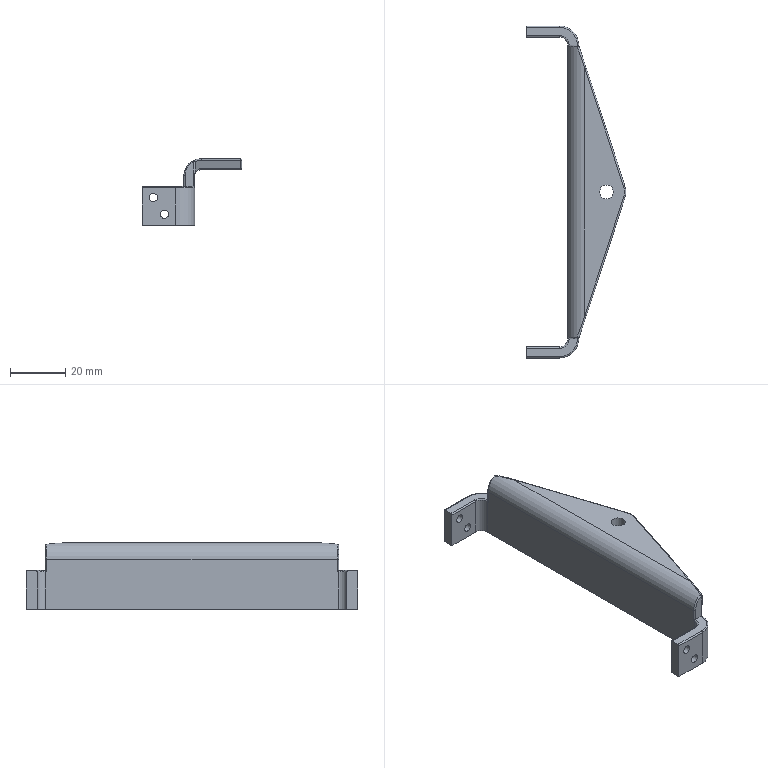Part | STEP file | 1-53.6 | 1 solid | 65 faces | box 36 x 120 x 24 mm | volume 15140 mm3 | cylinder 30 | plane 17 | torus 10 | spline 6 | sphere 2 | commonest cylinder face diameters 1 x18 3 x4 14 x3 6 x2 4 x1 5 x1